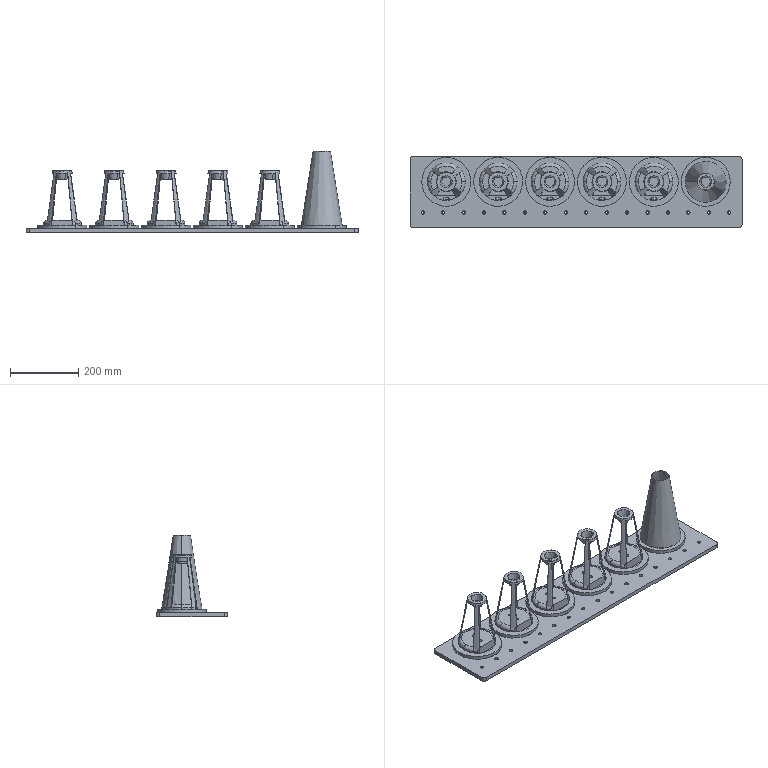Part | SolidWorks | 32 solids | 734 faces | box 975 x 210 x 240 mm | volume 4305889 mm3 | plane 354 | cylinder 266 | cone 96 | torus 18 | commonest cylinder face diameters 4 x72 5.5 x32 10 x32 3.3 x24 6.8 x24 8.4 x24